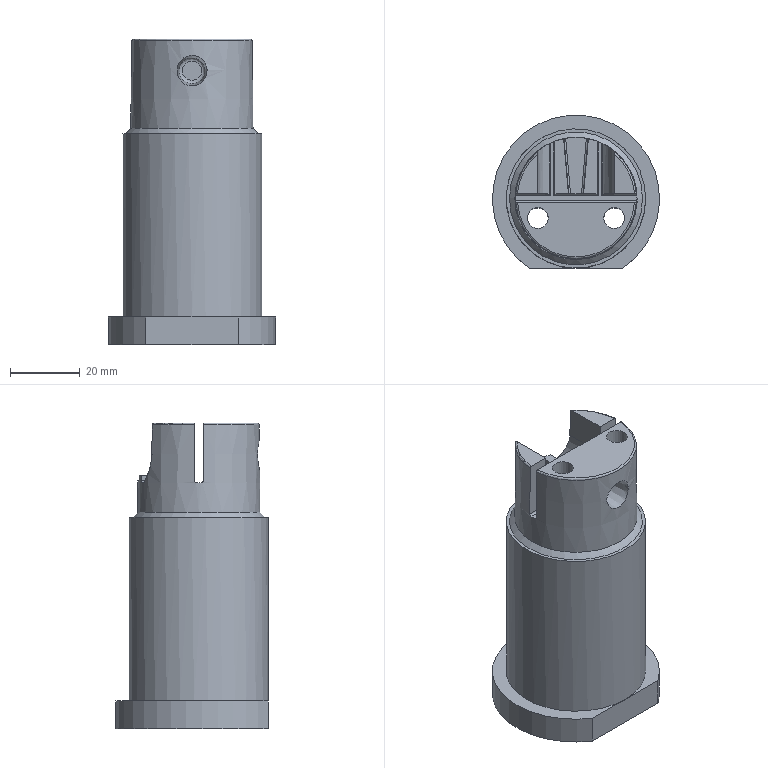Part | NX | features solid 2 | 1 solid | 47 faces | box 48 x 44 x 87.77 mm | volume 89878 mm3 | plane 21 | cylinder 17 | torus 4 | cone 3 | spline 2 | commonest cylinder face diameters 1.005 x8 1 x2 6 x2 22.11 x2 10 x1 40 x1
STEP:
#1=CARTESIAN_POINT('',(-13.266,-20.,-70.));
#2=VERTEX_POINT('',#1);
#3=CARTESIAN_POINT('',(13.266,-20.,-70.));
#4=VERTEX_POINT('',#3);
#5=CARTESIAN_POINT('',(0.,-20.,-70.));
#6=DIRECTION('',(1.,0.,0.));
#7=VECTOR('',#6,1000.);
#8=LINE('',#5,#7);
#9=EDGE_CURVE('',#2,#4,#8,.T.);
#10=ORIENTED_EDGE('',*,*,#9,.F.);
#11=CARTESIAN_POINT('',(0.,0.,-70.));
#12=DIRECTION('',(0.,0.,-1.));
#13=DIRECTION('',(-1.,0.,0.));
#14=AXIS2_PLACEMENT_3D('',#11,#12,#13);
#15=CIRCLE('',#14,24.);
#16=EDGE_CURVE('',#2,#4,#15,.T.);
#17=ORIENTED_EDGE('',*,*,#16,.T.);
#18=EDGE_LOOP('',(#10,#17));
#19=FACE_BOUND('',#18,.T.);
#20=CARTESIAN_POINT('',(7.98,-5.66,-70.));
#21=VERTEX_POINT('',#20);
#22=CARTESIAN_POINT('',(10.98,-5.66,-70.));
#23=DIRECTION('',(0.,0.,-1.));
#24=DIRECTION('',(-1.,0.,0.));
#25=AXIS2_PLACEMENT_3D('',#22,#23,#24);
#26=CIRCLE('',#25,3.);
#27=EDGE_CURVE('',#21,#21,#26,.T.);
#28=ORIENTED_EDGE('',*,*,#27,.F.);
#29=EDGE_LOOP('',(#28));
#30=FACE_BOUND('',#29,.T.);
#31=CARTESIAN_POINT('',(-13.98,-5.66,-70.));
#32=VERTEX_POINT('',#31);
#33=CARTESIAN_POINT('',(-10.98,-5.66,-70.));
#34=DIRECTION('',(0.,0.,-1.));
#35=DIRECTION('',(-1.,0.,0.));
#36=AXIS2_PLACEMENT_3D('',#33,#34,#35);
#37=CIRCLE('',#36,3.);
#38=EDGE_CURVE('',#32,#32,#37,.T.);
#39=ORIENTED_EDGE('',*,*,#38,.F.);
#40=EDGE_LOOP('',(#39));
#41=FACE_BOUND('',#40,.T.);
#42=CARTESIAN_POINT('',(-5.,7.,-70.));
#43=VERTEX_POINT('',#42);
#44=CARTESIAN_POINT('',(0.,7.,-70.));
#45=DIRECTION('',(0.,0.,-1.));
#46=DIRECTION('',(-1.,0.,0.));
#47=AXIS2_PLACEMENT_3D('',#44,#45,#46);
#48=CIRCLE('',#47,5.);
#49=EDGE_CURVE('',#43,#43,#48,.F.);
#50=ORIENTED_EDGE('',*,*,#49,.T.);
#51=EDGE_LOOP('',(#50));
#52=FACE_BOUND('',#51,.T.);
#53=CARTESIAN_POINT('',(0.,0.,-70.));
#54=DIRECTION('',(0.,0.,-1.));
#55=DIRECTION('',(-1.,0.,0.));
#56=AXIS2_PLACEMENT_3D('',#53,#54,#55);
#57=PLANE('',#56);
#58=ADVANCED_FACE('',(#19,#30,#41,#52),#57,.T.);
#59=CARTESIAN_POINT('',(0.,-20.,-62.));
#60=VERTEX_POINT('',#59);
#61=CARTESIAN_POINT('',(0.,0.,-62.));
#62=DIRECTION('',(0.,0.,-1.));
#63=DIRECTION('',(-1.,0.,0.));
#64=AXIS2_PLACEMENT_3D('',#61,#62,#63);
#65=CIRCLE('',#64,20.);
#66=EDGE_CURVE('',#60,#60,#65,.F.);
#67=ORIENTED_EDGE('',*,*,#66,.T.);
#68=EDGE_LOOP('',(#67));
#69=FACE_BOUND('',#68,.T.);
#70=CARTESIAN_POINT('',(20.,0.,-9.365));
#71=VERTEX_POINT('',#70);
#72=CARTESIAN_POINT('',(0.,0.,-9.365));
#73=DIRECTION('',(0.,0.,1.));
#74=DIRECTION('',(1.,0.,0.));
#75=AXIS2_PLACEMENT_3D('',#72,#73,#74);
#76=CIRCLE('',#75,20.);
#77=EDGE_CURVE('',#71,#71,#76,.F.);
#78=ORIENTED_EDGE('',*,*,#77,.T.);
#79=EDGE_LOOP('',(#78));
#80=FACE_BOUND('',#79,.T.);
#81=CARTESIAN_POINT('',(0.,0.,-104.365));
#82=DIRECTION('',(0.,0.,1.));
#83=DIRECTION('',(1.,0.,0.));
#84=AXIS2_PLACEMENT_3D('',#81,#82,#83);
#85=CYLINDRICAL_SURFACE('',#84,20.);
#86=ADVANCED_FACE('',(#69,#80),#85,.T.);
#87=CARTESIAN_POINT('',(0.,-9.452,11.49));
#88=VERTEX_POINT('',#87);
#89=CARTESIAN_POINT('',(0.,-9.452,8.725));
#90=DIRECTION('',(0.,1.,0.));
#91=DIRECTION('',(0.,0.,1.));
#92=AXIS2_PLACEMENT_3D('',#89,#90,#91);
#93=CIRCLE('',#92,2.764);
#94=EDGE_CURVE('',#88,#88,#93,.F.);
#95=ORIENTED_EDGE('',*,*,#94,.T.);
#96=EDGE_LOOP('',(#95));
#97=FACE_BOUND('',#96,.T.);
#98=CARTESIAN_POINT('',(0.,-9.452,8.725));
#99=DIRECTION('',(0.,1.,0.));
#100=DIRECTION('',(0.,0.,1.));
#101=AXIS2_PLACEMENT_3D('',#98,#99,#100);
#102=PLANE('',#101);
#103=ADVANCED_FACE('',(#97),#102,.F.);
#104=CARTESIAN_POINT('',(0.,-10.364,12.486));
#105=VERTEX_POINT('',#104);
#106=CARTESIAN_POINT('',(0.,-10.364,8.725));
#107=DIRECTION('',(0.,1.,0.));
#108=DIRECTION('',(0.,0.,1.));
#109=AXIS2_PLACEMENT_3D('',#106,#107,#108);
#110=CIRCLE('',#109,3.761);
#111=EDGE_CURVE('',#105,#105,#110,.T.);
#112=ORIENTED_EDGE('',*,*,#111,.F.);
#113=EDGE_LOOP('',(#112));
#114=FACE_BOUND('',#113,.T.);
#115=ORIENTED_EDGE('',*,*,#94,.F.);
#116=EDGE_LOOP('',(#115));
#117=FACE_BOUND('',#116,.T.);
#118=CARTESIAN_POINT('',(0.,-10.452,8.725));
#119=DIRECTION('',(0.,1.,0.));
#120=DIRECTION('',(0.,0.,1.));
#121=AXIS2_PLACEMENT_3D('',#118,#119,#120);
#122=TOROIDAL_SURFACE('',#121,2.764,1.);
#123=ADVANCED_FACE('',(#114,#117),#122,.F.);
#124=CARTESIAN_POINT('',(-11.055,12.72,17.77));
#125=VERTEX_POINT('',#124);
#126=CARTESIAN_POINT('',(-11.055,1.256,17.77));
#127=VERTEX_POINT('',#126);
#128=CARTESIAN_POINT('',(-11.055,1.256,17.77));
#129=DIRECTION('',(0.,1.,0.));
#130=VECTOR('',#129,1000.);
#131=LINE('',#128,#130);
#132=EDGE_CURVE('',#125,#127,#131,.F.);
#133=ORIENTED_EDGE('',*,*,#132,.F.);
#134=CARTESIAN_POINT('',(-16.806,1.256,17.77));
#135=VERTEX_POINT('',#134);
#136=CARTESIAN_POINT('',(0.,0.,17.77));
#137=DIRECTION('',(0.,0.,1.));
#138=DIRECTION('',(-0.656,0.7548,0.));
#139=AXIS2_PLACEMENT_3D('',#136,#137,#138);
#140=CIRCLE('',#139,16.853);
#141=EDGE_CURVE('',#135,#125,#140,.F.);
#142=ORIENTED_EDGE('',*,*,#141,.F.);
#143=CARTESIAN_POINT('',(-11.055,1.256,17.77));
#144=DIRECTION('',(-1.,0.,0.));
#145=VECTOR('',#144,1000.);
#146=LINE('',#143,#145);
#147=EDGE_CURVE('',#135,#127,#146,.F.);
#148=ORIENTED_EDGE('',*,*,#147,.T.);
#149=EDGE_LOOP('',(#133,#142,#148));
#150=FACE_BOUND('',#149,.T.);
#151=CARTESIAN_POINT('',(0.,0.,17.77));
#152=DIRECTION('',(0.,0.,-1.));
#153=DIRECTION('',(1.,0.,0.));
#154=AXIS2_PLACEMENT_3D('',#151,#152,#153);
#155=PLANE('',#154);
#156=ADVANCED_FACE('',(#150),#155,.F.);
#157=CARTESIAN_POINT('',(-13.98,-5.66,17.77));
#158=VERTEX_POINT('',#157);
#159=CARTESIAN_POINT('',(-10.98,-5.66,17.77));
#160=DIRECTION('',(0.,0.,-1.));
#161=DIRECTION('',(-1.,0.,0.));
#162=AXIS2_PLACEMENT_3D('',#159,#160,#161);
#163=CIRCLE('',#162,3.);
#164=EDGE_CURVE('',#158,#158,#163,.T.);
#165=ORIENTED_EDGE('',*,*,#164,.T.);
#166=EDGE_LOOP('',(#165));
#167=FACE_BOUND('',#166,.T.);
#168=CARTESIAN_POINT('',(7.98,-5.66,17.77));
#169=VERTEX_POINT('',#168);
#170=CARTESIAN_POINT('',(10.98,-5.66,17.77));
#171=DIRECTION('',(0.,0.,-1.));
#172=DIRECTION('',(-1.,0.,0.));
#173=AXIS2_PLACEMENT_3D('',#170,#171,#172);
#174=CIRCLE('',#173,3.);
#175=EDGE_CURVE('',#169,#169,#174,.T.);
#176=ORIENTED_EDGE('',*,*,#175,.T.);
#177=EDGE_LOOP('',(#176));
#178=FACE_BOUND('',#177,.T.);
#179=CARTESIAN_POINT('',(-16.806,-1.256,17.77));
#180=VERTEX_POINT('',#179);
#181=CARTESIAN_POINT('',(16.806,-1.256,17.77));
#182=VERTEX_POINT('',#181);
#183=CARTESIAN_POINT('',(16.806,-1.256,17.77));
#184=DIRECTION('',(-1.,0.,0.));
#185=VECTOR('',#184,1000.);
#186=LINE('',#183,#185);
#187=EDGE_CURVE('',#180,#182,#186,.F.);
#188=ORIENTED_EDGE('',*,*,#187,.F.);
#189=CARTESIAN_POINT('',(0.,0.,17.77));
#190=DIRECTION('',(0.,0.,1.));
#191=DIRECTION('',(-0.9972,-0.07454,0.));
#192=AXIS2_PLACEMENT_3D('',#189,#190,#191);
#193=CIRCLE('',#192,16.853);
#194=EDGE_CURVE('',#182,#180,#193,.F.);
#195=ORIENTED_EDGE('',*,*,#194,.F.);
#196=EDGE_LOOP('',(#188,#195));
#197=FACE_BOUND('',#196,.T.);
#198=CARTESIAN_POINT('',(0.,0.,17.77));
#199=DIRECTION('',(0.,0.,-1.));
#200=DIRECTION('',(1.,0.,0.));
#201=AXIS2_PLACEMENT_3D('',#198,#199,#200);
#202=PLANE('',#201);
#203=ADVANCED_FACE('',(#167,#178,#197),#202,.F.);
#204=CARTESIAN_POINT('',(11.055,1.256,17.77));
#205=VERTEX_POINT('',#204);
#206=CARTESIAN_POINT('',(16.806,1.256,17.77));
#207=VERTEX_POINT('',#206);
#208=CARTESIAN_POINT('',(16.806,1.256,17.77));
#209=DIRECTION('',(-1.,0.,0.));
#210=VECTOR('',#209,1000.);
#211=LINE('',#208,#210);
#212=EDGE_CURVE('',#205,#207,#211,.F.);
#213=ORIENTED_EDGE('',*,*,#212,.T.);
#214=CARTESIAN_POINT('',(11.055,12.72,17.77));
#215=VERTEX_POINT('',#214);
#216=CARTESIAN_POINT('',(0.,0.,17.77));
#217=DIRECTION('',(0.,0.,1.));
#218=DIRECTION('',(0.9972,0.07454,0.));
#219=AXIS2_PLACEMENT_3D('',#216,#217,#218);
#220=CIRCLE('',#219,16.853);
#221=EDGE_CURVE('',#215,#207,#220,.F.);
#222=ORIENTED_EDGE('',*,*,#221,.F.);
#223=CARTESIAN_POINT('',(11.055,12.72,17.77));
#224=DIRECTION('',(0.,-1.,0.));
#225=VECTOR('',#224,1000.);
#226=LINE('',#223,#225);
#227=EDGE_CURVE('',#205,#215,#226,.F.);
#228=ORIENTED_EDGE('',*,*,#227,.F.);
#229=EDGE_LOOP('',(#213,#222,#228));
#230=FACE_BOUND('',#229,.T.);
#231=CARTESIAN_POINT('',(0.,0.,17.77));
#232=DIRECTION('',(0.,0.,-1.));
#233=DIRECTION('',(1.,0.,0.));
#234=AXIS2_PLACEMENT_3D('',#231,#232,#233);
#235=PLANE('',#234);
#236=ADVANCED_FACE('',(#230),#235,.F.);
#237=CARTESIAN_POINT('',(-6.03,1.256,1.188));
#238=VERTEX_POINT('',#237);
#239=CARTESIAN_POINT('',(6.03,1.256,1.188));
#240=VERTEX_POINT('',#239);
#241=CARTESIAN_POINT('',(6.03,1.256,1.188));
#242=DIRECTION('',(-1.,0.,0.));
#243=VECTOR('',#242,1000.);
#244=LINE('',#241,#243);
#245=EDGE_CURVE('',#238,#240,#244,.F.);
#246=ORIENTED_EDGE('',*,*,#245,.F.);
#247=CARTESIAN_POINT('',(-6.532,0.7538,0.6852));
#248=VERTEX_POINT('',#247);
#249=CARTESIAN_POINT('',(-6.532,0.7538,1.188));
#250=DIRECTION('',(-0.7071,0.7071,0.));
#251=DIRECTION('',(-0.7071,-0.7071,0.));
#252=AXIS2_PLACEMENT_3D('',#249,#250,#251);
#253=ELLIPSE('',#252,0.7106,0.5025);
#254=EDGE_CURVE('',#248,#238,#253,.F.);
#255=ORIENTED_EDGE('',*,*,#254,.F.);
#256=CARTESIAN_POINT('',(6.532,0.7538,0.6852));
#257=VERTEX_POINT('',#256);
#258=CARTESIAN_POINT('',(6.532,0.7538,0.6852));
#259=DIRECTION('',(-1.,0.,0.));
#260=VECTOR('',#259,1000.);
#261=LINE('',#258,#260);
#262=EDGE_CURVE('',#248,#257,#261,.F.);
#263=ORIENTED_EDGE('',*,*,#262,.T.);
#264=CARTESIAN_POINT('',(6.532,0.7538,1.188));
#265=DIRECTION('',(-0.7071,-0.7071,0.));
#266=DIRECTION('',(-0.7071,0.7071,0.));
#267=AXIS2_PLACEMENT_3D('',#264,#265,#266);
#268=ELLIPSE('',#267,0.7106,0.5025);
#269=EDGE_CURVE('',#240,#257,#268,.T.);
#270=ORIENTED_EDGE('',*,*,#269,.F.);
#271=EDGE_LOOP('',(#246,#255,#263,#270));
#272=FACE_BOUND('',#271,.T.);
#273=CARTESIAN_POINT('',(196.261,0.7538,1.188));
#274=DIRECTION('',(-1.,0.,0.));
#275=DIRECTION('',(0.,-1.,0.));
#276=AXIS2_PLACEMENT_3D('',#273,#274,#275);
#277=CYLINDRICAL_SURFACE('',#276,0.5025);
#278=ADVANCED_FACE('',(#272),#277,.F.);
#279=CARTESIAN_POINT('',(-2.07,1.256,1.656));
#280=VERTEX_POINT('',#279);
#281=CARTESIAN_POINT('',(-1.57,1.256,1.2));
#282=VERTEX_POINT('',#281);
#283=CARTESIAN_POINT('',(-1.57,1.256,1.7));
#284=DIRECTION('',(0.,1.,0.));
#285=DIRECTION('',(1.,0.,0.));
#286=AXIS2_PLACEMENT_3D('',#283,#284,#285);
#287=ELLIPSE('',#286,0.5019,0.5);
#288=EDGE_CURVE('',#280,#282,#287,.F.);
#289=ORIENTED_EDGE('',*,*,#288,.F.);
#290=CARTESIAN_POINT('',(-2.188,1.256,3.004));
#291=VERTEX_POINT('',#290);
#292=CARTESIAN_POINT('',(-2.03,1.256,1.2));
#293=DIRECTION('',(-0.08749,0.,0.9962));
#294=VECTOR('',#293,1000.);
#295=LINE('',#292,#294);
#296=EDGE_CURVE('',#280,#291,#295,.T.);
#297=ORIENTED_EDGE('',*,*,#296,.T.);
#298=CARTESIAN_POINT('',(-6.03,1.256,3.004));
#299=VERTEX_POINT('',#298);
#300=CARTESIAN_POINT('',(0.,1.256,3.004));
#301=DIRECTION('',(-1.,0.,0.));
#302=VECTOR('',#301,1000.);
#303=LINE('',#300,#302);
#304=EDGE_CURVE('',#291,#299,#303,.T.);
#305=ORIENTED_EDGE('',*,*,#304,.T.);
#306=CARTESIAN_POINT('',(-6.03,1.256,1.188));
#307=DIRECTION('',(0.,0.,1.));
#308=VECTOR('',#307,1000.);
#309=LINE('',#306,#308);
#310=EDGE_CURVE('',#299,#238,#309,.F.);
#311=ORIENTED_EDGE('',*,*,#310,.T.);
#312=ORIENTED_EDGE('',*,*,#245,.T.);
#313=CARTESIAN_POINT('',(6.03,1.256,3.004));
#314=VERTEX_POINT('',#313);
#315=CARTESIAN_POINT('',(6.03,1.256,1.188));
#316=DIRECTION('',(0.,0.,1.));
#317=VECTOR('',#316,1000.);
#318=LINE('',#315,#317);
#319=EDGE_CURVE('',#314,#240,#318,.F.);
#320=ORIENTED_EDGE('',*,*,#319,.F.);
#321=CARTESIAN_POINT('',(2.188,1.256,3.004));
#322=VERTEX_POINT('',#321);
#323=CARTESIAN_POINT('',(0.,1.256,3.004));
#324=DIRECTION('',(-1.,0.,0.));
#325=VECTOR('',#324,1000.);
#326=LINE('',#323,#325);
#327=EDGE_CURVE('',#314,#322,#326,.T.);
#328=ORIENTED_EDGE('',*,*,#327,.T.);
#329=CARTESIAN_POINT('',(2.07,1.256,1.656));
#330=VERTEX_POINT('',#329);
#331=CARTESIAN_POINT('',(1.997,1.256,0.8247));
#332=DIRECTION('',(0.08749,0.,0.9962));
#333=VECTOR('',#332,1000.);
#334=LINE('',#331,#333);
#335=EDGE_CURVE('',#330,#322,#334,.T.);
#336=ORIENTED_EDGE('',*,*,#335,.F.);
#337=CARTESIAN_POINT('',(1.57,1.256,1.2));
#338=VERTEX_POINT('',#337);
#339=CARTESIAN_POINT('',(1.57,1.256,1.7));
#340=DIRECTION('',(0.,1.,0.));
#341=DIRECTION('',(1.,0.,0.));
#342=AXIS2_PLACEMENT_3D('',#339,#340,#341);
#343=ELLIPSE('',#342,0.5019,0.5);
#344=EDGE_CURVE('',#338,#330,#343,.F.);
#345=ORIENTED_EDGE('',*,*,#344,.F.);
#346=CARTESIAN_POINT('',(0.,1.256,1.2));
#347=DIRECTION('',(1.,0.,0.));
#348=VECTOR('',#347,1000.);
#349=LINE('',#346,#348);
#350=EDGE_CURVE('',#282,#338,#349,.T.);
#351=ORIENTED_EDGE('',*,*,#350,.F.);
#352=EDGE_LOOP('',(#289,#297,#305,#311,#312,#320,#328,#336,#345,#351));
#353=FACE_BOUND('',#352,.T.);
#354=CARTESIAN_POINT('',(-18.15,1.256,17.77));
#355=DIRECTION('',(0.,1.,0.));
#356=DIRECTION('',(-1.,0.,0.));
#357=AXIS2_PLACEMENT_3D('',#354,#355,#356);
#358=PLANE('',#357);
#359=ADVANCED_FACE('',(#353),#358,.F.);
#360=ORIENTED_EDGE('',*,*,#111,.T.);
#361=EDGE_LOOP('',(#360));
#362=FACE_BOUND('',#361,.T.);
#363=CARTESIAN_POINT('',(-3.148,-17.17,5.715));
#364=VERTEX_POINT('',#363);
#365=CARTESIAN_POINT('',(-0.1207,-17.607,3.863));
#366=CARTESIAN_POINT('',(-3.495,-17.166,5.395));
#367=CARTESIAN_POINT('',(-4.79,-16.745,8.843));
#368=CARTESIAN_POINT('',(-3.323,-17.147,12.223));
#369=CARTESIAN_POINT('',(0.1224,-17.523,13.581));
#370=CARTESIAN_POINT('',(3.495,-17.107,12.048));
#371=CARTESIAN_POINT('',(4.79,-16.747,8.598));
#372=CARTESIAN_POINT('',(3.32,-17.21,5.218));
#373=CARTESIAN_POINT('',(-0.1207,-17.607,3.863));
#374=CARTESIAN_POINT('',(-3.495,-17.166,5.395));
#375=CARTESIAN_POINT('',(-4.79,-16.745,8.843));
#376=B_SPLINE_CURVE_WITH_KNOTS('',3,(#365,#366,#367,#368,#369,#370,#371,#372,#373,#374,#375),.UNSPECIFIED.,.T.,.F.,(1,1,1,1,1,1,1,1,1,1,1,1,1,1,1),(-0.01025,-0.006833,-0.003417,0.,0.003417,0.006833,0.01025,0.01367,0.01708,0.0205,0.02392,0.02733,0.03075,0.03417,0.03758),.UNSPECIFIED.);
#377=EDGE_CURVE('',#364,#364,#376,.T.);
#378=ORIENTED_EDGE('',*,*,#377,.F.);
#379=EDGE_LOOP('',(#378));
#380=FACE_BOUND('',#379,.T.);
#381=CARTESIAN_POINT('',(0.,-13.8,8.725));
#382=DIRECTION('',(0.,-1.,0.));
#383=DIRECTION('',(0.,0.,1.));
#384=AXIS2_PLACEMENT_3D('',#381,#382,#383);
#385=CONICAL_SURFACE('',#384,4.061,0.08727);
#386=ADVANCED_FACE('',(#362,#380),#385,.F.);
#387=ORIENTED_EDGE('',*,*,#335,.T.);
#388=CARTESIAN_POINT('',(3.558,17.115,2.805));
#389=VERTEX_POINT('',#388);
#390=CARTESIAN_POINT('',(2.188,1.256,3.004));
#391=CARTESIAN_POINT('',(2.645,6.543,2.937));
#392=CARTESIAN_POINT('',(3.102,11.829,2.87));
#393=CARTESIAN_POINT('',(3.558,17.115,2.805));
#394=B_SPLINE_CURVE_WITH_KNOTS('',3,(#390,#391,#392,#393),.UNSPECIFIED.,.F.,.F.,(4,4),(0.,0.01592),.UNSPECIFIED.);
#395=EDGE_CURVE('',#322,#389,#394,.T.);
#396=ORIENTED_EDGE('',*,*,#395,.T.);
#397=CARTESIAN_POINT('',(3.46,17.146,1.656));
#398=VERTEX_POINT('',#397);
#399=CARTESIAN_POINT('',(-1.775,0.1553,-41.03));
#400=DIRECTION('',(0.9924,-0.08682,-0.08716));
#401=DIRECTION('',(-0.08682,0.007596,-0.9962));
#402=AXIS2_PLACEMENT_3D('',#399,#400,#401);
#403=ELLIPSE('',#402,204.965,17.775);
#404=EDGE_CURVE('',#398,#389,#403,.T.);
#405=ORIENTED_EDGE('',*,*,#404,.F.);
#406=CARTESIAN_POINT('',(2.07,1.253,1.656));
#407=DIRECTION('',(0.08716,0.9962,0.));
#408=VECTOR('',#407,1000.);
#409=LINE('',#406,#408);
#410=EDGE_CURVE('',#398,#330,#409,.F.);
#411=ORIENTED_EDGE('',*,*,#410,.T.);
#412=EDGE_LOOP('',(#387,#396,#405,#411));
#413=FACE_BOUND('',#412,.T.);
#414=CARTESIAN_POINT('',(2.03,1.256,1.2));
#415=DIRECTION('',(0.9924,-0.08682,-0.08716));
#416=DIRECTION('',(-0.08749,0.,-0.9962));
#417=AXIS2_PLACEMENT_3D('',#414,#415,#416);
#418=PLANE('',#417);
#419=ADVANCED_FACE('',(#413),#418,.F.);
#420=ORIENTED_EDGE('',*,*,#344,.T.);
#421=ORIENTED_EDGE('',*,*,#410,.F.);
#422=CARTESIAN_POINT('',(2.969,17.242,1.2));
#423=VERTEX_POINT('',#422);
#424=CARTESIAN_POINT('',(3.46,17.146,1.656));
#425=CARTESIAN_POINT('',(3.439,17.152,1.407));
#426=CARTESIAN_POINT('',(3.215,17.199,1.2));
#427=CARTESIAN_POINT('',(2.969,17.242,1.2));
#428=B_SPLINE_CURVE_WITH_KNOTS('',3,(#424,#425,#426,#427),.UNSPECIFIED.,.F.,.F.,(4,4),(0.,0.0007397),.UNSPECIFIED.);
#429=EDGE_CURVE('',#398,#423,#428,.T.);
#430=ORIENTED_EDGE('',*,*,#429,.T.);
#431=CARTESIAN_POINT('',(2.263,9.171,1.2));
#432=DIRECTION('',(0.08716,0.9962,0.));
#433=VECTOR('',#432,1000.);
#434=LINE('',#431,#433);
#435=EDGE_CURVE('',#338,#423,#434,.T.);
#436=ORIENTED_EDGE('',*,*,#435,.F.);
#437=EDGE_LOOP('',(#420,#421,#430,#436));
#438=FACE_BOUND('',#437,.T.);
#439=CARTESIAN_POINT('',(1.574,1.296,1.7));
#440=DIRECTION('',(0.08716,0.9962,0.));
#441=DIRECTION('',(-0.9962,0.08716,0.));
#442=AXIS2_PLACEMENT_3D('',#439,#440,#441);
#443=CYLINDRICAL_SURFACE('',#442,0.5);
#444=ADVANCED_FACE('',(#438),#443,.F.);
#445=ORIENTED_EDGE('',*,*,#350,.T.);
#446=ORIENTED_EDGE('',*,*,#435,.T.);
#447=CARTESIAN_POINT('',(-2.969,17.242,1.2));
#448=VERTEX_POINT('',#447);
#449=CARTESIAN_POINT('',(0.,0.,1.2));
#450=DIRECTION('',(0.,0.,-1.));
#451=DIRECTION('',(-1.,0.,0.));
#452=AXIS2_PLACEMENT_3D('',#449,#450,#451);
#453=CIRCLE('',#452,17.495);
#454=EDGE_CURVE('',#448,#423,#453,.T.);
#455=ORIENTED_EDGE('',*,*,#454,.F.);
#456=CARTESIAN_POINT('',(-2.263,9.171,1.2));
#457=DIRECTION('',(0.08716,-0.9962,0.));
#458=VECTOR('',#457,1000.);
#459=LINE('',#456,#458);
#460=EDGE_CURVE('',#448,#282,#459,.T.);
#461=ORIENTED_EDGE('',*,*,#460,.T.);
#462=EDGE_LOOP('',(#445,#446,#455,#461));
#463=FACE_BOUND('',#462,.T.);
#464=CARTESIAN_POINT('',(0.,9.369,1.2));
#465=DIRECTION('',(0.,0.,-1.));
#466=DIRECTION('',(-1.,0.,0.));
#467=AXIS2_PLACEMENT_3D('',#464,#465,#466);
#468=PLANE('',#467);
#469=ADVANCED_FACE('',(#463),#468,.F.);
#470=CARTESIAN_POINT('',(-3.46,17.146,1.656));
#471=VERTEX_POINT('',#470);
#472=CARTESIAN_POINT('',(-2.969,17.242,1.2));
#473=CARTESIAN_POINT('',(-3.215,17.199,1.2));
#474=CARTESIAN_POINT('',(-3.439,17.152,1.407));
#475=CARTESIAN_POINT('',(-3.46,17.146,1.656));
#476=B_SPLINE_CURVE_WITH_KNOTS('',3,(#472,#473,#474,#475),.UNSPECIFIED.,.F.,.F.,(4,4),(0.,0.0007398),.UNSPECIFIED.);
#477=EDGE_CURVE('',#448,#471,#476,.T.);
#478=ORIENTED_EDGE('',*,*,#477,.T.);
#479=CARTESIAN_POINT('',(-2.07,1.253,1.656));
#480=DIRECTION('',(0.08716,-0.9962,0.));
#481=VECTOR('',#480,1000.);
#482=LINE('',#479,#481);
#483=EDGE_CURVE('',#280,#471,#482,.F.);
#484=ORIENTED_EDGE('',*,*,#483,.F.);
#485=ORIENTED_EDGE('',*,*,#288,.T.);
#486=ORIENTED_EDGE('',*,*,#460,.F.);
#487=EDGE_LOOP('',(#478,#484,#485,#486));
#488=FACE_BOUND('',#487,.T.);
#489=CARTESIAN_POINT('',(-1.574,1.296,1.7));
#490=DIRECTION('',(0.08716,-0.9962,0.));
#491=DIRECTION('',(0.9962,0.08716,0.));
#492=AXIS2_PLACEMENT_3D('',#489,#490,#491);
#493=CYLINDRICAL_SURFACE('',#492,0.5);
#494=ADVANCED_FACE('',(#488),#493,.F.);
#495=CARTESIAN_POINT('',(-3.558,17.115,2.805));
#496=VERTEX_POINT('',#495);
#497=CARTESIAN_POINT('',(1.775,0.1553,-41.03));
#498=DIRECTION('',(-0.9924,-0.08682,-0.08716));
#499=DIRECTION('',(0.08682,0.007596,-0.9962));
#500=AXIS2_PLACEMENT_3D('',#497,#498,#499);
#501=ELLIPSE('',#500,204.965,17.775);
#502=EDGE_CURVE('',#496,#471,#501,.T.);
#503=ORIENTED_EDGE('',*,*,#502,.F.);
#504=CARTESIAN_POINT('',(-3.558,17.115,2.805));
#505=CARTESIAN_POINT('',(-3.102,11.829,2.87));
#506=CARTESIAN_POINT('',(-2.645,6.543,2.937));
#507=CARTESIAN_POINT('',(-2.188,1.256,3.004));
#508=B_SPLINE_CURVE_WITH_KNOTS('',3,(#504,#505,#506,#507),.UNSPECIFIED.,.F.,.F.,(4,4),(0.0003674,0.01629),.UNSPECIFIED.);
#509=EDGE_CURVE('',#496,#291,#508,.T.);
#510=ORIENTED_EDGE('',*,*,#509,.T.);
#511=ORIENTED_EDGE('',*,*,#296,.F.);
#512=ORIENTED_EDGE('',*,*,#483,.T.);
#513=EDGE_LOOP('',(#503,#510,#511,#512));
#514=FACE_BOUND('',#513,.T.);
#515=CARTESIAN_POINT('',(-2.03,1.256,1.2));
#516=DIRECTION('',(-0.9924,-0.08682,-0.08716));
#517=DIRECTION('',(-0.08749,0.,0.9962));
#518=AXIS2_PLACEMENT_3D('',#515,#516,#517);
#519=PLANE('',#518);
#520=ADVANCED_FACE('',(#514),#519,.F.);
#521=ORIENTED_EDGE('',*,*,#509,.F.);
#522=CARTESIAN_POINT('',(-6.03,16.408,2.813));
#523=VERTEX_POINT('',#522);
#524=CARTESIAN_POINT('',(-6.03,16.408,2.813));
#525=CARTESIAN_POINT('',(-5.217,16.707,2.81));
#526=CARTESIAN_POINT('',(-4.393,16.942,2.807));
#527=CARTESIAN_POINT('',(-3.558,17.115,2.805));
#528=B_SPLINE_CURVE_WITH_KNOTS('',3,(#524,#525,#526,#527),.UNSPECIFIED.,.F.,.F.,(4,4),(0.,0.002557),.UNSPECIFIED.);
#529=EDGE_CURVE('',#523,#496,#528,.T.);
#530=ORIENTED_EDGE('',*,*,#529,.F.);
#531=CARTESIAN_POINT('',(-6.03,1.256,3.004));
#532=CARTESIAN_POINT('',(-6.03,6.307,2.94));
#533=CARTESIAN_POINT('',(-6.03,11.358,2.876));
#534=CARTESIAN_POINT('',(-6.03,16.408,2.813));
#535=B_SPLINE_CURVE_WITH_KNOTS('',3,(#531,#532,#533,#534),.UNSPECIFIED.,.F.,.F.,(4,4),(0.,1.),.PIECEWISE_BEZIER_KNOTS.);
#536=EDGE_CURVE('',#523,#299,#535,.F.);
#537=ORIENTED_EDGE('',*,*,#536,.T.);
#538=ORIENTED_EDGE('',*,*,#304,.F.);
#539=EDGE_LOOP('',(#521,#530,#537,#538));
#540=FACE_BOUND('',#539,.T.);
#541=CARTESIAN_POINT('',(-2.165,17.21,2.803));
#542=CARTESIAN_POINT('',(-6.03,17.21,2.803));
#543=CARTESIAN_POINT('',(-2.165,16.943,2.807));
#544=CARTESIAN_POINT('',(-6.03,16.943,2.807));
#545=CARTESIAN_POINT('',(-2.165,11.625,2.873));
#546=CARTESIAN_POINT('',(-6.03,11.625,2.873));
#547=CARTESIAN_POINT('',(-2.165,6.307,2.94));
#548=CARTESIAN_POINT('',(-6.03,6.307,2.94));
#549=CARTESIAN_POINT('',(-2.165,1.256,3.004));
#550=CARTESIAN_POINT('',(-6.03,1.256,3.004));
#551=B_SPLINE_SURFACE_WITH_KNOTS('',3,1,((#541,#542),(#543,#544),(#545,#546),(#547,#548),(#549,#550)),.SURF_OF_LINEAR_EXTRUSION.,.F.,.F.,.F.,(4,1,4),(2,2),(-0.05294,0.,1.),(0.6795,1.),.UNSPECIFIED.);
#552=ADVANCED_FACE('',(#540),#551,.F.);
#553=CARTESIAN_POINT('',(-6.03,16.423,1.188));
#554=VERTEX_POINT('',#553);
#555=CARTESIAN_POINT('',(-6.03,16.408,2.813));
#556=CARTESIAN_POINT('',(-6.03,16.413,2.272));
#557=CARTESIAN_POINT('',(-6.03,16.418,1.73));
#558=CARTESIAN_POINT('',(-6.03,16.423,1.188));
#559=B_SPLINE_CURVE_WITH_KNOTS('',3,(#555,#556,#557,#558),.UNSPECIFIED.,.F.,.F.,(4,4),(0.,1.),.PIECEWISE_BEZIER_KNOTS.);
#560=EDGE_CURVE('',#554,#523,#559,.F.);
#561=ORIENTED_EDGE('',*,*,#560,.F.);
#562=CARTESIAN_POINT('',(-6.03,1.256,1.188));
#563=DIRECTION('',(0.,1.,0.));
#564=VECTOR('',#563,1000.);
#565=LINE('',#562,#564);
#566=EDGE_CURVE('',#554,#238,#565,.F.);
#567=ORIENTED_EDGE('',*,*,#566,.T.);
#568=ORIENTED_EDGE('',*,*,#310,.F.);
#569=ORIENTED_EDGE('',*,*,#536,.F.);
#570=EDGE_LOOP('',(#561,#567,#568,#569));
#571=FACE_BOUND('',#570,.T.);
#572=CARTESIAN_POINT('',(-6.03,0.,-0.5405));
#573=DIRECTION('',(1.,0.,0.));
#574=DIRECTION('',(0.,0.,-1.));
#575=AXIS2_PLACEMENT_3D('',#572,#573,#574);
#576=PLANE('',#575);
#577=ADVANCED_FACE('',(#571),#576,.F.);
#578=CARTESIAN_POINT('',(-6.532,16.235,0.6852));
#579=VERTEX_POINT('',#578);
#580=CARTESIAN_POINT('',(-6.03,16.423,1.188));
#581=CARTESIAN_POINT('',(-6.03,16.426,0.9127));
#582=CARTESIAN_POINT('',(-6.278,16.337,0.6852));
#583=CARTESIAN_POINT('',(-6.532,16.235,0.6852));
#584=B_SPLINE_CURVE_WITH_KNOTS('',3,(#580,#581,#582,#583),.UNSPECIFIED.,.F.,.F.,(4,4),(0.,0.0008129),.UNSPECIFIED.);
#585=EDGE_CURVE('',#579,#554,#584,.F.);
#586=ORIENTED_EDGE('',*,*,#585,.F.);
#587=CARTESIAN_POINT('',(-6.532,16.235,0.6852));
#588=DIRECTION('',(0.,-1.,0.));
#589=VECTOR('',#588,1000.);
#590=LINE('',#587,#589);
#591=EDGE_CURVE('',#248,#579,#590,.F.);
#592=ORIENTED_EDGE('',*,*,#591,.F.);
#593=ORIENTED_EDGE('',*,*,#254,.T.);
#594=ORIENTED_EDGE('',*,*,#566,.F.);
#595=EDGE_LOOP('',(#586,#592,#593,#594));
#596=FACE_BOUND('',#595,.T.);
#597=CARTESIAN_POINT('',(-6.532,-212.801,1.188));
#598=DIRECTION('',(0.,1.,0.));
#599=DIRECTION('',(-1.,0.,0.));
#600=AXIS2_PLACEMENT_3D('',#597,#598,#599);
#601=CYLINDRICAL_SURFACE('',#600,0.5025);
#602=ADVANCED_FACE('',(#596),#601,.F.);
#603=CARTESIAN_POINT('',(-7.737,15.695,0.8288));
#604=VERTEX_POINT('',#603);
#605=CARTESIAN_POINT('',(-7.385,15.865,0.6852));
#606=VERTEX_POINT('',#605);
#607=CARTESIAN_POINT('',(-7.385,15.865,0.6852));
#608=CARTESIAN_POINT('',(-7.515,15.805,0.6852));
#609=CARTESIAN_POINT('',(-7.64,15.744,0.7343));
#610=CARTESIAN_POINT('',(-7.737,15.695,0.8288));
#611=B_SPLINE_CURVE_WITH_KNOTS('',3,(#607,#608,#609,#610),.UNSPECIFIED.,.F.,.F.,(4,4),(0.,0.0004236),.UNSPECIFIED.);
#612=EDGE_CURVE('',#604,#606,#611,.F.);
#613=ORIENTED_EDGE('',*,*,#612,.F.);
#614=CARTESIAN_POINT('',(-7.737,1.105,0.8288));
#615=VERTEX_POINT('',#614);
#616=CARTESIAN_POINT('',(-7.737,1.105,0.8288));
#617=DIRECTION('',(0.,1.,0.));
#618=VECTOR('',#617,1000.);
#619=LINE('',#616,#618);
#620=EDGE_CURVE('',#604,#615,#619,.F.);
#621=ORIENTED_EDGE('',*,*,#620,.T.);
#622=CARTESIAN_POINT('',(-7.385,0.7538,0.6852));
#623=VERTEX_POINT('',#622);
#624=CARTESIAN_POINT('',(-7.385,0.7538,1.188));
#625=DIRECTION('',(-0.7071,-0.7071,0.));
#626=DIRECTION('',(0.7071,-0.7071,0.));
#627=AXIS2_PLACEMENT_3D('',#624,#625,#626);
#628=ELLIPSE('',#627,0.7106,0.5025);
#629=EDGE_CURVE('',#623,#615,#628,.F.);
#630=ORIENTED_EDGE('',*,*,#629,.F.);
#631=CARTESIAN_POINT('',(-7.385,15.865,0.6852));
#632=DIRECTION('',(0.,-1.,0.));
#633=VECTOR('',#632,1000.);
#634=LINE('',#631,#633);
#635=EDGE_CURVE('',#623,#606,#634,.F.);
#636=ORIENTED_EDGE('',*,*,#635,.T.);
#637=EDGE_LOOP('',(#613,#621,#630,#636));
#638=FACE_BOUND('',#637,.T.);
#639=CARTESIAN_POINT('',(-7.385,227.196,1.188));
#640=DIRECTION('',(0.,-1.,0.));
#641=DIRECTION('',(0.6999,0.,0.7143));
#642=AXIS2_PLACEMENT_3D('',#639,#640,#641);
#643=CYLINDRICAL_SURFACE('',#642,0.5025);
#644=ADVANCED_FACE('',(#638),#643,.F.);
#645=CARTESIAN_POINT('',(-11.055,1.256,8.725));
#646=VERTEX_POINT('',#645);
#647=CARTESIAN_POINT('',(-11.055,13.475,8.725));
#648=VERTEX_POINT('',#647);
#649=CARTESIAN_POINT('',(-11.055,13.475,8.725));
#650=DIRECTION('',(0.,-1.,0.));
#651=VECTOR('',#650,1000.);
#652=LINE('',#649,#651);
#653=EDGE_CURVE('',#646,#648,#652,.F.);
#654=ORIENTED_EDGE('',*,*,#653,.F.);
#655=CARTESIAN_POINT('',(-8.087,1.256,1.188));
#656=VERTEX_POINT('',#655);
#657=CARTESIAN_POINT('',(0.,1.256,8.725));
#658=DIRECTION('',(0.,-1.,0.));
#659=DIRECTION('',(-1.,0.,0.));
#660=AXIS2_PLACEMENT_3D('',#657,#658,#659);
#661=CIRCLE('',#660,11.055);
#662=EDGE_CURVE('',#656,#646,#661,.F.);
#663=ORIENTED_EDGE('',*,*,#662,.F.);
#664=CARTESIAN_POINT('',(-7.737,1.105,0.8288));
#665=CARTESIAN_POINT('',(-7.841,1.21,0.9308));
#666=CARTESIAN_POINT('',(-7.965,1.256,1.057));
#667=CARTESIAN_POINT('',(-8.087,1.256,1.188));
#668=B_SPLINE_CURVE_WITH_KNOTS('',3,(#664,#665,#666,#667),.UNSPECIFIED.,.F.,.F.,(4,4),(0.,0.0005294),.UNSPECIFIED.);
#669=EDGE_CURVE('',#656,#615,#668,.F.);
#670=ORIENTED_EDGE('',*,*,#669,.T.);
#671=ORIENTED_EDGE('',*,*,#620,.F.);
#672=CARTESIAN_POINT('',(-7.737,15.695,0.8288));
#673=CARTESIAN_POINT('',(-8.765,15.178,1.836));
#674=CARTESIAN_POINT('',(-10.401,14.089,4.2));
#675=CARTESIAN_POINT('',(-11.055,13.492,7.191));
#676=CARTESIAN_POINT('',(-11.055,13.475,8.725));
#677=B_SPLINE_CURVE_WITH_KNOTS('',3,(#672,#673,#674,#675,#676),.UNSPECIFIED.,.F.,.F.,(4,1,4),(0.,0.004531,0.009061),.UNSPECIFIED.);
#678=EDGE_CURVE('',#648,#604,#677,.F.);
#679=ORIENTED_EDGE('',*,*,#678,.F.);
#680=EDGE_LOOP('',(#654,#663,#670,#671,#679));
#681=FACE_BOUND('',#680,.T.);
#682=CARTESIAN_POINT('',(0.,0.,8.725));
#683=DIRECTION('',(0.,-1.,0.));
#684=DIRECTION('',(0.,0.,-1.));
#685=AXIS2_PLACEMENT_3D('',#682,#683,#684);
#686=CYLINDRICAL_SURFACE('',#685,11.055);
#687=ADVANCED_FACE('',(#681),#686,.F.);
#688=CARTESIAN_POINT('',(-11.055,13.379,17.272));
#689=VERTEX_POINT('',#688);
#690=CARTESIAN_POINT('',(-11.055,13.379,17.272));
#691=CARTESIAN_POINT('',(-11.055,13.389,16.324));
#692=CARTESIAN_POINT('',(-11.055,13.411,14.427));
#693=CARTESIAN_POINT('',(-11.055,13.443,11.578));
#694=CARTESIAN_POINT('',(-11.055,13.464,9.676));
#695=CARTESIAN_POINT('',(-11.055,13.475,8.725));
#696=B_SPLINE_CURVE_WITH_KNOTS('',3,(#690,#691,#692,#693,#694,#695),.UNSPECIFIED.,.F.,.F.,(4,1,1,4),(0.,0.3333,0.6667,1.),.QUASI_UNIFORM_KNOTS.);
#697=EDGE_CURVE('',#648,#689,#696,.F.);
#698=ORIENTED_EDGE('',*,*,#697,.T.);
#699=CARTESIAN_POINT('',(-11.055,12.72,17.77));
#700=CARTESIAN_POINT('',(-11.055,13.026,17.77));
#701=CARTESIAN_POINT('',(-11.055,13.375,17.58));
#702=CARTESIAN_POINT('',(-11.055,13.379,17.272));
#703=B_SPLINE_CURVE_WITH_KNOTS('',3,(#699,#700,#701,#702),.UNSPECIFIED.,.F.,.F.,(4,4),(0.,0.000907),.UNSPECIFIED.);
#704=EDGE_CURVE('',#689,#125,#703,.F.);
#705=ORIENTED_EDGE('',*,*,#704,.T.);
#706=ORIENTED_EDGE('',*,*,#132,.T.);
#707=CARTESIAN_POINT('',(-11.055,1.256,17.77));
#708=DIRECTION('',(0.,0.,-1.));
#709=VECTOR('',#708,1000.);
#710=LINE('',#707,#709);
#711=EDGE_CURVE('',#646,#127,#710,.F.);
#712=ORIENTED_EDGE('',*,*,#711,.F.);
#713=ORIENTED_EDGE('',*,*,#653,.T.);
#714=EDGE_LOOP('',(#698,#705,#706,#712,#713));
#715=FACE_BOUND('',#714,.T.);
#716=CARTESIAN_POINT('',(-11.055,0.,19.558));
#717=DIRECTION('',(-1.,0.,0.));
#718=DIRECTION('',(0.,0.,1.));
#719=AXIS2_PLACEMENT_3D('',#716,#717,#718);
#720=PLANE('',#719);
#721=ADVANCED_FACE('',(#715),#720,.F.);
#722=CARTESIAN_POINT('',(-17.31,1.256,17.272));
#723=VERTEX_POINT('',#722);
#724=CARTESIAN_POINT('',(0.,0.,17.272));
#725=DIRECTION('',(0.,0.,1.));
#726=DIRECTION('',(-0.637,0.7709,0.));
#727=AXIS2_PLACEMENT_3D('',#724,#725,#726);
#728=CIRCLE('',#727,17.355);
#729=EDGE_CURVE('',#723,#689,#728,.F.);
#730=ORIENTED_EDGE('',*,*,#729,.F.);
#731=CARTESIAN_POINT('',(-17.31,1.256,17.272));
#732=CARTESIAN_POINT('',(-17.307,1.256,17.536));
#733=CARTESIAN_POINT('',(-17.07,1.256,17.77));
#734=CARTESIAN_POINT('',(-16.806,1.256,17.77));
#735=B_SPLINE_CURVE_WITH_KNOTS('',3,(#731,#732,#733,#734),.UNSPECIFIED.,.F.,.F.,(4,4),(0.,0.0007817),.UNSPECIFIED.);
#736=EDGE_CURVE('',#135,#723,#735,.F.);
#737=ORIENTED_EDGE('',*,*,#736,.F.);
#738=ORIENTED_EDGE('',*,*,#141,.T.);
#739=ORIENTED_EDGE('',*,*,#704,.F.);
#740=EDGE_LOOP('',(#730,#737,#738,#739));
#741=FACE_BOUND('',#740,.T.);
#742=CARTESIAN_POINT('',(0.,0.,17.268));
#743=DIRECTION('',(0.,0.,-1.));
#744=DIRECTION('',(-0.0009333,1.,0.));
#745=AXIS2_PLACEMENT_3D('',#742,#743,#744);
#746=TOROIDAL_SURFACE('',#745,16.853,0.5025);
#747=ADVANCED_FACE('',(#741),#746,.T.);
#748=CARTESIAN_POINT('',(-17.45,1.256,1.188));
#749=VERTEX_POINT('',#748);
#750=CARTESIAN_POINT('',(-17.45,1.256,1.188));
#751=DIRECTION('',(0.008749,0.,1.));
#752=VECTOR('',#751,1000.);
#753=LINE('',#750,#752);
#754=EDGE_CURVE('',#723,#749,#753,.F.);
#755=ORIENTED_EDGE('',*,*,#754,.T.);
#756=CARTESIAN_POINT('',(-17.45,1.256,1.188));
#757=DIRECTION('',(1.,0.,0.));
#758=VECTOR('',#757,1000.);
#759=LINE('',#756,#758);
#760=EDGE_CURVE('',#656,#749,#759,.F.);
#761=ORIENTED_EDGE('',*,*,#760,.F.);
#762=ORIENTED_EDGE('',*,*,#662,.T.);
#763=ORIENTED_EDGE('',*,*,#711,.T.);
#764=ORIENTED_EDGE('',*,*,#147,.F.);
#765=ORIENTED_EDGE('',*,*,#736,.T.);
#766=EDGE_LOOP('',(#755,#761,#762,#763,#764,#765));
#767=FACE_BOUND('',#766,.T.);
#768=CARTESIAN_POINT('',(-18.15,1.256,17.77));
#769=DIRECTION('',(0.,1.,0.));
#770=DIRECTION('',(-1.,0.,0.));
#771=AXIS2_PLACEMENT_3D('',#768,#769,#770);
#772=PLANE('',#771);
#773=ADVANCED_FACE('',(#767),#772,.F.);
#774=CARTESIAN_POINT('',(-17.484,0.7538,0.6852));
#775=VERTEX_POINT('',#774);
#776=CARTESIAN_POINT('',(-17.45,1.256,1.188));
#777=CARTESIAN_POINT('',(-17.453,1.256,0.922));
#778=CARTESIAN_POINT('',(-17.472,1.019,0.6852));
#779=CARTESIAN_POINT('',(-17.484,0.7538,0.6852));
#780=B_SPLINE_CURVE_WITH_KNOTS('',3,(#776,#777,#778,#779),.UNSPECIFIED.,.F.,.F.,(4,4),(0.,0.0007857),.UNSPECIFIED.);
#781=EDGE_CURVE('',#775,#749,#780,.F.);
#782=ORIENTED_EDGE('',*,*,#781,.F.);
#783=CARTESIAN_POINT('',(-17.484,0.7538,0.6852));
#784=DIRECTION('',(1.,0.,0.));
#785=VECTOR('',#784,1000.);
#786=LINE('',#783,#785);
#787=EDGE_CURVE('',#623,#775,#786,.F.);
#788=ORIENTED_EDGE('',*,*,#787,.F.);
#789=ORIENTED_EDGE('',*,*,#629,.T.);
#790=ORIENTED_EDGE('',*,*,#669,.F.);
#791=ORIENTED_EDGE('',*,*,#760,.T.);
#792=EDGE_LOOP('',(#782,#788,#789,#790,#791));
#793=FACE_BOUND('',#792,.T.);
#794=CARTESIAN_POINT('',(-193.862,0.7538,1.188));
#795=DIRECTION('',(1.,0.,0.));
#796=DIRECTION('',(0.,0.,1.));
#797=AXIS2_PLACEMENT_3D('',#794,#795,#796);
#798=CYLINDRICAL_SURFACE('',#797,0.5025);
#799=ADVANCED_FACE('',(#793),#798,.F.);
#800=ORIENTED_EDGE('',*,*,#194,.T.);
#801=CARTESIAN_POINT('',(-17.31,-1.256,17.272));
#802=VERTEX_POINT('',#801);
#803=CARTESIAN_POINT('',(-16.806,-1.256,17.77));
#804=CARTESIAN_POINT('',(-17.07,-1.256,17.77));
#805=CARTESIAN_POINT('',(-17.307,-1.256,17.536));
#806=CARTESIAN_POINT('',(-17.31,-1.256,17.272));
#807=B_SPLINE_CURVE_WITH_KNOTS('',3,(#803,#804,#805,#806),.UNSPECIFIED.,.F.,.F.,(4,4),(0.,0.0007817),.UNSPECIFIED.);
#808=EDGE_CURVE('',#802,#180,#807,.F.);
#809=ORIENTED_EDGE('',*,*,#808,.F.);
#810=CARTESIAN_POINT('',(17.31,-1.256,17.272));
#811=VERTEX_POINT('',#810);
#812=CARTESIAN_POINT('',(0.,0.,17.272));
#813=DIRECTION('',(0.,0.,1.));
#814=DIRECTION('',(-0.9974,-0.07239,0.));
#815=AXIS2_PLACEMENT_3D('',#812,#813,#814);
#816=CIRCLE('',#815,17.355);
#817=EDGE_CURVE('',#811,#802,#816,.F.);
#818=ORIENTED_EDGE('',*,*,#817,.F.);
#819=CARTESIAN_POINT('',(17.31,-1.256,17.272));
#820=CARTESIAN_POINT('',(17.307,-1.256,17.536));
#821=CARTESIAN_POINT('',(17.07,-1.256,17.77));
#822=CARTESIAN_POINT('',(16.806,-1.256,17.77));
#823=B_SPLINE_CURVE_WITH_KNOTS('',3,(#819,#820,#821,#822),.UNSPECIFIED.,.F.,.F.,(4,4),(0.,0.0007817),.UNSPECIFIED.);
#824=EDGE_CURVE('',#182,#811,#823,.F.);
#825=ORIENTED_EDGE('',*,*,#824,.F.);
#826=EDGE_LOOP('',(#800,#809,#818,#825));
#827=FACE_BOUND('',#826,.T.);
#828=CARTESIAN_POINT('',(0.,0.,17.268));
#829=DIRECTION('',(0.,0.,-1.));
#830=DIRECTION('',(0.0009333,-1.,0.));
#831=AXIS2_PLACEMENT_3D('',#828,#829,#830);
#832=TOROIDAL_SURFACE('',#831,16.853,0.5025);
#833=ADVANCED_FACE('',(#827),#832,.T.);
#834=CARTESIAN_POINT('',(-17.45,-1.256,1.188));
#835=VERTEX_POINT('',#834);
#836=CARTESIAN_POINT('',(17.45,-1.256,1.188));
#837=VERTEX_POINT('',#836);
#838=CARTESIAN_POINT('',(17.45,-1.256,1.188));
#839=DIRECTION('',(-1.,0.,0.));
#840=VECTOR('',#839,1000.);
#841=LINE('',#838,#840);
#842=EDGE_CURVE('',#835,#837,#841,.F.);
#843=ORIENTED_EDGE('',*,*,#842,.F.);
#844=CARTESIAN_POINT('',(-17.31,-1.256,17.272));
#845=DIRECTION('',(-0.008749,0.,-1.));
#846=VECTOR('',#845,1000.);
#847=LINE('',#844,#846);
#848=EDGE_CURVE('',#835,#802,#847,.F.);
#849=ORIENTED_EDGE('',*,*,#848,.T.);
#850=ORIENTED_EDGE('',*,*,#808,.T.);
#851=ORIENTED_EDGE('',*,*,#187,.T.);
#852=ORIENTED_EDGE('',*,*,#824,.T.);
#853=CARTESIAN_POINT('',(17.45,-1.256,1.188));
#854=DIRECTION('',(-0.008749,0.,1.));
#855=VECTOR('',#854,1000.);
#856=LINE('',#853,#855);
#857=EDGE_CURVE('',#811,#837,#856,.F.);
#858=ORIENTED_EDGE('',*,*,#857,.T.);
#859=EDGE_LOOP('',(#843,#849,#850,#851,#852,#858));
#860=FACE_BOUND('',#859,.T.);
#861=CARTESIAN_POINT('',(18.281,-1.256,17.77));
#862=DIRECTION('',(0.,-1.,0.));
#863=DIRECTION('',(1.,0.,0.));
#864=AXIS2_PLACEMENT_3D('',#861,#862,#863);
#865=PLANE('',#864);
#866=ADVANCED_FACE('',(#860),#865,.F.);
#867=CARTESIAN_POINT('',(-17.484,-0.7538,0.6852));
#868=VERTEX_POINT('',#867);
#869=CARTESIAN_POINT('',(17.484,-0.7538,0.6852));
#870=VERTEX_POINT('',#869);
#871=CARTESIAN_POINT('',(17.484,-0.7538,0.6852));
#872=DIRECTION('',(-1.,0.,0.));
#873=VECTOR('',#872,1000.);
#874=LINE('',#871,#873);
#875=EDGE_CURVE('',#868,#870,#874,.F.);
#876=ORIENTED_EDGE('',*,*,#875,.F.);
#877=CARTESIAN_POINT('',(-17.484,-0.7538,0.6852));
#878=CARTESIAN_POINT('',(-17.472,-1.019,0.6852));
#879=CARTESIAN_POINT('',(-17.453,-1.256,0.922));
#880=CARTESIAN_POINT('',(-17.45,-1.256,1.188));
#881=B_SPLINE_CURVE_WITH_KNOTS('',3,(#877,#878,#879,#880),.UNSPECIFIED.,.F.,.F.,(4,4),(0.,0.0007857),.UNSPECIFIED.);
#882=EDGE_CURVE('',#835,#868,#881,.F.);
#883=ORIENTED_EDGE('',*,*,#882,.F.);
#884=ORIENTED_EDGE('',*,*,#842,.T.);
#885=CARTESIAN_POINT('',(17.45,-1.256,1.188));
#886=CARTESIAN_POINT('',(17.453,-1.256,0.922));
#887=CARTESIAN_POINT('',(17.472,-1.019,0.6852));
#888=CARTESIAN_POINT('',(17.484,-0.7538,0.6852));
#889=B_SPLINE_CURVE_WITH_KNOTS('',3,(#885,#886,#887,#888),.UNSPECIFIED.,.F.,.F.,(4,4),(0.,0.0007857),.UNSPECIFIED.);
#890=EDGE_CURVE('',#870,#837,#889,.F.);
#891=ORIENTED_EDGE('',*,*,#890,.F.);
#892=EDGE_LOOP('',(#876,#883,#884,#891));
#893=FACE_BOUND('',#892,.T.);
#894=CARTESIAN_POINT('',(196.261,-0.7538,1.188));
#895=DIRECTION('',(-1.,0.,0.));
#896=DIRECTION('',(0.,0.,1.));
#897=AXIS2_PLACEMENT_3D('',#894,#895,#896);
#898=CYLINDRICAL_SURFACE('',#897,0.5025);
#899=ADVANCED_FACE('',(#893),#898,.F.);
#900=CARTESIAN_POINT('',(17.45,1.256,1.188));
#901=VERTEX_POINT('',#900);
#902=CARTESIAN_POINT('',(17.484,0.7538,0.6852));
#903=VERTEX_POINT('',#902);
#904=CARTESIAN_POINT('',(17.484,0.7538,0.6852));
#905=CARTESIAN_POINT('',(17.472,1.019,0.6852));
#906=CARTESIAN_POINT('',(17.453,1.256,0.922));
#907=CARTESIAN_POINT('',(17.45,1.256,1.188));
#908=B_SPLINE_CURVE_WITH_KNOTS('',3,(#904,#905,#906,#907),.UNSPECIFIED.,.F.,.F.,(4,4),(0.,0.0007857),.UNSPECIFIED.);
#909=EDGE_CURVE('',#901,#903,#908,.F.);
#910=ORIENTED_EDGE('',*,*,#909,.F.);
#911=CARTESIAN_POINT('',(8.087,1.256,1.188));
#912=VERTEX_POINT('',#911);
#913=CARTESIAN_POINT('',(8.087,1.256,1.188));
#914=DIRECTION('',(1.,0.,0.));
#915=VECTOR('',#914,1000.);
#916=LINE('',#913,#915);
#917=EDGE_CURVE('',#901,#912,#916,.F.);
#918=ORIENTED_EDGE('',*,*,#917,.T.);
#919=CARTESIAN_POINT('',(7.737,1.105,0.8288));
#920=VERTEX_POINT('',#919);
#921=CARTESIAN_POINT('',(8.087,1.256,1.188));
#922=CARTESIAN_POINT('',(7.965,1.256,1.057));
#923=CARTESIAN_POINT('',(7.841,1.21,0.9307));
#924=CARTESIAN_POINT('',(7.737,1.105,0.8288));
#925=B_SPLINE_CURVE_WITH_KNOTS('',3,(#921,#922,#923,#924),.UNSPECIFIED.,.F.,.F.,(4,4),(0.,0.0005283),.UNSPECIFIED.);
#926=EDGE_CURVE('',#920,#912,#925,.F.);
#927=ORIENTED_EDGE('',*,*,#926,.F.);
#928=CARTESIAN_POINT('',(7.385,0.7538,0.6852));
#929=VERTEX_POINT('',#928);
#930=CARTESIAN_POINT('',(7.385,0.7538,1.188));
#931=DIRECTION('',(0.7071,-0.7071,0.));
#932=DIRECTION('',(0.7071,0.7071,0.));
#933=AXIS2_PLACEMENT_3D('',#930,#931,#932);
#934=ELLIPSE('',#933,0.7106,0.5025);
#935=EDGE_CURVE('',#929,#920,#934,.T.);
#936=ORIENTED_EDGE('',*,*,#935,.F.);
#937=CARTESIAN_POINT('',(7.385,0.7538,0.6852));
#938=DIRECTION('',(1.,0.,0.));
#939=VECTOR('',#938,1000.);
#940=LINE('',#937,#939);
#941=EDGE_CURVE('',#903,#929,#940,.F.);
#942=ORIENTED_EDGE('',*,*,#941,.F.);
#943=EDGE_LOOP('',(#910,#918,#927,#936,#942));
#944=FACE_BOUND('',#943,.T.);
#945=CARTESIAN_POINT('',(-193.862,0.7538,1.188));
#946=DIRECTION('',(1.,0.,0.));
#947=DIRECTION('',(0.,0.,1.));
#948=AXIS2_PLACEMENT_3D('',#945,#946,#947);
#949=CYLINDRICAL_SURFACE('',#948,0.5025);
#950=ADVANCED_FACE('',(#944),#949,.F.);
#951=CARTESIAN_POINT('',(11.055,1.256,8.725));
#952=VERTEX_POINT('',#951);
#953=CARTESIAN_POINT('',(0.,1.256,8.725));
#954=DIRECTION('',(0.,-1.,0.));
#955=DIRECTION('',(0.7315,0.,-0.6818));
#956=AXIS2_PLACEMENT_3D('',#953,#954,#955);
#957=CIRCLE('',#956,11.055);
#958=EDGE_CURVE('',#952,#912,#957,.F.);
#959=ORIENTED_EDGE('',*,*,#958,.T.);
#960=ORIENTED_EDGE('',*,*,#917,.F.);
#961=CARTESIAN_POINT('',(17.31,1.256,17.272));
#962=VERTEX_POINT('',#961);
#963=CARTESIAN_POINT('',(17.31,1.256,17.272));
#964=DIRECTION('',(0.008749,0.,-1.));
#965=VECTOR('',#964,1000.);
#966=LINE('',#963,#965);
#967=EDGE_CURVE('',#901,#962,#966,.F.);
#968=ORIENTED_EDGE('',*,*,#967,.T.);
#969=CARTESIAN_POINT('',(16.806,1.256,17.77));
#970=CARTESIAN_POINT('',(17.07,1.256,17.77));
#971=CARTESIAN_POINT('',(17.307,1.256,17.536));
#972=CARTESIAN_POINT('',(17.31,1.256,17.272));
#973=B_SPLINE_CURVE_WITH_KNOTS('',3,(#969,#970,#971,#972),.UNSPECIFIED.,.F.,.F.,(4,4),(0.,0.0007817),.UNSPECIFIED.);
#974=EDGE_CURVE('',#962,#207,#973,.F.);
#975=ORIENTED_EDGE('',*,*,#974,.T.);
#976=ORIENTED_EDGE('',*,*,#212,.F.);
#977=CARTESIAN_POINT('',(11.055,1.256,17.77));
#978=DIRECTION('',(0.,0.,-1.));
#979=VECTOR('',#978,1000.);
#980=LINE('',#977,#979);
#981=EDGE_CURVE('',#952,#205,#980,.F.);
#982=ORIENTED_EDGE('',*,*,#981,.F.);
#983=EDGE_LOOP('',(#959,#960,#968,#975,#976,#982));
#984=FACE_BOUND('',#983,.T.);
#985=CARTESIAN_POINT('',(-18.15,1.256,17.77));
#986=DIRECTION('',(0.,1.,0.));
#987=DIRECTION('',(-1.,0.,0.));
#988=AXIS2_PLACEMENT_3D('',#985,#986,#987);
#989=PLANE('',#988);
#990=ADVANCED_FACE('',(#984),#989,.F.);
#991=CARTESIAN_POINT('',(11.055,13.379,17.272));
#992=VERTEX_POINT('',#991);
#993=CARTESIAN_POINT('',(0.,0.,17.272));
#994=DIRECTION('',(0.,0.,1.));
#995=DIRECTION('',(0.9974,0.07239,0.));
#996=AXIS2_PLACEMENT_3D('',#993,#994,#995);
#997=CIRCLE('',#996,17.355);
#998=EDGE_CURVE('',#992,#962,#997,.F.);
#999=ORIENTED_EDGE('',*,*,#998,.F.);
#1000=CARTESIAN_POINT('',(11.055,13.379,17.272));
#1001=CARTESIAN_POINT('',(11.055,13.375,17.58));
#1002=CARTESIAN_POINT('',(11.055,13.026,17.77));
#1003=CARTESIAN_POINT('',(11.055,12.72,17.77));
#1004=B_SPLINE_CURVE_WITH_KNOTS('',3,(#1000,#1001,#1002,#1003),.UNSPECIFIED.,.F.,.F.,(4,4),(0.,0.0009086),.UNSPECIFIED.);
#1005=EDGE_CURVE('',#215,#992,#1004,.F.);
#1006=ORIENTED_EDGE('',*,*,#1005,.F.);
#1007=ORIENTED_EDGE('',*,*,#221,.T.);
#1008=ORIENTED_EDGE('',*,*,#974,.F.);
#1009=EDGE_LOOP('',(#999,#1006,#1007,#1008));
#1010=FACE_BOUND('',#1009,.T.);
#1011=CARTESIAN_POINT('',(0.,0.,17.268));
#1012=DIRECTION('',(0.,0.,-1.));
#1013=DIRECTION('',(-0.0009333,1.,0.));
#1014=AXIS2_PLACEMENT_3D('',#1011,#1012,#1013);
#1015=TOROIDAL_SURFACE('',#1014,16.853,0.5025);
#1016=ADVANCED_FACE('',(#1010),#1015,.T.);
#1017=ORIENTED_EDGE('',*,*,#227,.T.);
#1018=ORIENTED_EDGE('',*,*,#1005,.T.);
#1019=CARTESIAN_POINT('',(11.055,13.475,8.725));
#1020=VERTEX_POINT('',#1019);
#1021=CARTESIAN_POINT('',(11.055,13.475,8.725));
#1022=CARTESIAN_POINT('',(11.055,13.464,9.676));
#1023=CARTESIAN_POINT('',(11.055,13.443,11.578));
#1024=CARTESIAN_POINT('',(11.055,13.411,14.427));
#1025=CARTESIAN_POINT('',(11.055,13.389,16.324));
#1026=CARTESIAN_POINT('',(11.055,13.379,17.272));
#1027=B_SPLINE_CURVE_WITH_KNOTS('',3,(#1021,#1022,#1023,#1024,#1025,#1026),.UNSPECIFIED.,.F.,.F.,(4,1,1,4),(0.,0.3333,0.6667,1.),.QUASI_UNIFORM_KNOTS.);
#1028=EDGE_CURVE('',#992,#1020,#1027,.F.);
#1029=ORIENTED_EDGE('',*,*,#1028,.T.);
#1030=CARTESIAN_POINT('',(11.055,13.475,8.725));
#1031=DIRECTION('',(0.,-1.,0.));
#1032=VECTOR('',#1031,1000.);
#1033=LINE('',#1030,#1032);
#1034=EDGE_CURVE('',#952,#1020,#1033,.F.);
#1035=ORIENTED_EDGE('',*,*,#1034,.F.);
#1036=ORIENTED_EDGE('',*,*,#981,.T.);
#1037=EDGE_LOOP('',(#1017,#1018,#1029,#1035,#1036));
#1038=FACE_BOUND('',#1037,.T.);
#1039=CARTESIAN_POINT('',(11.055,0.,8.725));
#1040=DIRECTION('',(1.,0.,0.));
#1041=DIRECTION('',(0.,0.,-1.));
#1042=AXIS2_PLACEMENT_3D('',#1039,#1040,#1041);
#1043=PLANE('',#1042);
#1044=ADVANCED_FACE('',(#1038),#1043,.F.);
#1045=CARTESIAN_POINT('',(7.737,15.695,0.8288));
#1046=VERTEX_POINT('',#1045);
#1047=CARTESIAN_POINT('',(11.055,13.475,8.725));
#1048=CARTESIAN_POINT('',(11.055,13.51,5.656));
#1049=CARTESIAN_POINT('',(9.794,14.662,2.844));
#1050=CARTESIAN_POINT('',(7.737,15.695,0.8288));
#1051=B_SPLINE_CURVE_WITH_KNOTS('',3,(#1047,#1048,#1049,#1050),.UNSPECIFIED.,.F.,.F.,(4,4),(0.,0.009047),.UNSPECIFIED.);
#1052=EDGE_CURVE('',#1046,#1020,#1051,.F.);
#1053=ORIENTED_EDGE('',*,*,#1052,.F.);
#1054=CARTESIAN_POINT('',(7.737,15.695,0.8288));
#1055=DIRECTION('',(0.,-1.,0.));
#1056=VECTOR('',#1055,1000.);
#1057=LINE('',#1054,#1056);
#1058=EDGE_CURVE('',#920,#1046,#1057,.F.);
#1059=ORIENTED_EDGE('',*,*,#1058,.F.);
#1060=ORIENTED_EDGE('',*,*,#926,.T.);
#1061=ORIENTED_EDGE('',*,*,#958,.F.);
#1062=ORIENTED_EDGE('',*,*,#1034,.T.);
#1063=EDGE_LOOP('',(#1053,#1059,#1060,#1061,#1062));
#1064=FACE_BOUND('',#1063,.T.);
#1065=CARTESIAN_POINT('',(0.,0.,8.725));
#1066=DIRECTION('',(0.,-1.,0.));
#1067=DIRECTION('',(0.,0.,-1.));
#1068=AXIS2_PLACEMENT_3D('',#1065,#1066,#1067);
#1069=CYLINDRICAL_SURFACE('',#1068,11.055);
#1070=ADVANCED_FACE('',(#1064),#1069,.F.);
#1071=CARTESIAN_POINT('',(7.385,15.865,0.6852));
#1072=VERTEX_POINT('',#1071);
#1073=CARTESIAN_POINT('',(7.737,15.695,0.8288));
#1074=CARTESIAN_POINT('',(7.641,15.744,0.7345));
#1075=CARTESIAN_POINT('',(7.515,15.805,0.6852));
#1076=CARTESIAN_POINT('',(7.385,15.865,0.6852));
#1077=B_SPLINE_CURVE_WITH_KNOTS('',3,(#1073,#1074,#1075,#1076),.UNSPECIFIED.,.F.,.F.,(4,4),(0.,0.0004226),.UNSPECIFIED.);
#1078=EDGE_CURVE('',#1072,#1046,#1077,.F.);
#1079=ORIENTED_EDGE('',*,*,#1078,.F.);
#1080=CARTESIAN_POINT('',(7.385,0.7538,0.6852));
#1081=DIRECTION('',(0.,1.,0.));
#1082=VECTOR('',#1081,1000.);
#1083=LINE('',#1080,#1082);
#1084=EDGE_CURVE('',#1072,#929,#1083,.F.);
#1085=ORIENTED_EDGE('',*,*,#1084,.T.);
#1086=ORIENTED_EDGE('',*,*,#935,.T.);
#1087=ORIENTED_EDGE('',*,*,#1058,.T.);
#1088=EDGE_LOOP('',(#1079,#1085,#1086,#1087));
#1089=FACE_BOUND('',#1088,.T.);
#1090=CARTESIAN_POINT('',(7.385,-228.924,1.188));
#1091=DIRECTION('',(0.,1.,0.));
#1092=DIRECTION('',(-0.6999,0.,0.7143));
#1093=AXIS2_PLACEMENT_3D('',#1090,#1091,#1092);
#1094=CYLINDRICAL_SURFACE('',#1093,0.5025);
#1095=ADVANCED_FACE('',(#1089),#1094,.F.);
#1096=CARTESIAN_POINT('',(0.,0.,0.6852));
#1097=DIRECTION('',(0.,0.,-1.));
#1098=DIRECTION('',(-1.,0.,0.));
#1099=AXIS2_PLACEMENT_3D('',#1096,#1097,#1098);
#1100=CIRCLE('',#1099,17.5);
#1101=EDGE_CURVE('',#775,#868,#1100,.F.);
#1102=ORIENTED_EDGE('',*,*,#1101,.T.);
#1103=ORIENTED_EDGE('',*,*,#875,.T.);
#1104=CARTESIAN_POINT('',(0.,0.,0.6852));
#1105=DIRECTION('',(0.,0.,-1.));
#1106=DIRECTION('',(1.,0.,0.));
#1107=AXIS2_PLACEMENT_3D('',#1104,#1105,#1106);
#1108=CIRCLE('',#1107,17.5);
#1109=EDGE_CURVE('',#870,#903,#1108,.F.);
#1110=ORIENTED_EDGE('',*,*,#1109,.T.);
#1111=ORIENTED_EDGE('',*,*,#941,.T.);
#1112=ORIENTED_EDGE('',*,*,#1084,.F.);
#1113=CARTESIAN_POINT('',(6.532,16.235,0.6852));
#1114=VERTEX_POINT('',#1113);
#1115=CARTESIAN_POINT('',(0.,0.,0.6852));
#1116=DIRECTION('',(0.,0.,-1.));
#1117=DIRECTION('',(0.3733,0.9277,0.));
#1118=AXIS2_PLACEMENT_3D('',#1115,#1116,#1117);
#1119=CIRCLE('',#1118,17.5);
#1120=EDGE_CURVE('',#1072,#1114,#1119,.F.);
#1121=ORIENTED_EDGE('',*,*,#1120,.T.);
#1122=CARTESIAN_POINT('',(6.532,0.7538,0.6852));
#1123=DIRECTION('',(0.,1.,0.));
#1124=VECTOR('',#1123,1000.);
#1125=LINE('',#1122,#1124);
#1126=EDGE_CURVE('',#1114,#257,#1125,.F.);
#1127=ORIENTED_EDGE('',*,*,#1126,.T.);
#1128=ORIENTED_EDGE('',*,*,#262,.F.);
#1129=ORIENTED_EDGE('',*,*,#591,.T.);
#1130=CARTESIAN_POINT('',(0.,0.,0.6852));
#1131=DIRECTION('',(0.,0.,-1.));
#1132=DIRECTION('',(-0.422,0.9066,0.));
#1133=AXIS2_PLACEMENT_3D('',#1130,#1131,#1132);
#1134=CIRCLE('',#1133,17.5);
#1135=EDGE_CURVE('',#579,#606,#1134,.F.);
#1136=ORIENTED_EDGE('',*,*,#1135,.T.);
#1137=ORIENTED_EDGE('',*,*,#635,.F.);
#1138=ORIENTED_EDGE('',*,*,#787,.T.);
#1139=EDGE_LOOP('',(#1102,#1103,#1110,#1111,#1112,#1121,#1127,#1128,#1129,#1136,#1137,#1138));
#1140=FACE_BOUND('',#1139,.T.);
#1141=CARTESIAN_POINT('',(0.,0.,0.6852));
#1142=DIRECTION('',(0.,0.,-1.));
#1143=DIRECTION('',(0.,-1.,0.));
#1144=AXIS2_PLACEMENT_3D('',#1141,#1142,#1143);
#1145=PLANE('',#1144);
#1146=ADVANCED_FACE('',(#1140),#1145,.F.);
#1147=CARTESIAN_POINT('',(6.03,16.423,1.188));
#1148=VERTEX_POINT('',#1147);
#1149=CARTESIAN_POINT('',(6.532,16.235,0.6852));
#1150=CARTESIAN_POINT('',(6.278,16.337,0.6852));
#1151=CARTESIAN_POINT('',(6.03,16.426,0.9124));
#1152=CARTESIAN_POINT('',(6.03,16.423,1.188));
#1153=B_SPLINE_CURVE_WITH_KNOTS('',3,(#1149,#1150,#1151,#1152),.UNSPECIFIED.,.F.,.F.,(4,4),(0.,0.0008129),.UNSPECIFIED.);
#1154=EDGE_CURVE('',#1148,#1114,#1153,.F.);
#1155=ORIENTED_EDGE('',*,*,#1154,.F.);
#1156=CARTESIAN_POINT('',(6.03,16.423,1.188));
#1157=DIRECTION('',(0.,-1.,0.));
#1158=VECTOR('',#1157,1000.);
#1159=LINE('',#1156,#1158);
#1160=EDGE_CURVE('',#240,#1148,#1159,.F.);
#1161=ORIENTED_EDGE('',*,*,#1160,.F.);
#1162=ORIENTED_EDGE('',*,*,#269,.T.);
#1163=ORIENTED_EDGE('',*,*,#1126,.F.);
#1164=EDGE_LOOP('',(#1155,#1161,#1162,#1163));
#1165=FACE_BOUND('',#1164,.T.);
#1166=CARTESIAN_POINT('',(6.532,241.98,1.188));
#1167=DIRECTION('',(0.,-1.,0.));
#1168=DIRECTION('',(1.,0.,0.));
#1169=AXIS2_PLACEMENT_3D('',#1166,#1167,#1168);
#1170=CYLINDRICAL_SURFACE('',#1169,0.5025);
#1171=ADVANCED_FACE('',(#1165),#1170,.F.);
#1172=ORIENTED_EDGE('',*,*,#319,.T.);
#1173=ORIENTED_EDGE('',*,*,#1160,.T.);
#1174=CARTESIAN_POINT('',(6.03,16.408,2.813));
#1175=VERTEX_POINT('',#1174);
#1176=CARTESIAN_POINT('',(6.03,16.423,1.188));
#1177=CARTESIAN_POINT('',(6.03,16.418,1.73));
#1178=CARTESIAN_POINT('',(6.03,16.413,2.272));
#1179=CARTESIAN_POINT('',(6.03,16.408,2.813));
#1180=B_SPLINE_CURVE_WITH_KNOTS('',3,(#1176,#1177,#1178,#1179),.UNSPECIFIED.,.F.,.F.,(4,4),(0.,1.),.PIECEWISE_BEZIER_KNOTS.);
#1181=EDGE_CURVE('',#1175,#1148,#1180,.F.);
#1182=ORIENTED_EDGE('',*,*,#1181,.F.);
#1183=CARTESIAN_POINT('',(6.03,16.408,2.813));
#1184=CARTESIAN_POINT('',(6.03,11.358,2.876));
#1185=CARTESIAN_POINT('',(6.03,6.307,2.94));
#1186=CARTESIAN_POINT('',(6.03,1.256,3.004));
#1187=B_SPLINE_CURVE_WITH_KNOTS('',3,(#1183,#1184,#1185,#1186),.UNSPECIFIED.,.F.,.F.,(4,4),(0.,1.),.PIECEWISE_BEZIER_KNOTS.);
#1188=EDGE_CURVE('',#314,#1175,#1187,.F.);
#1189=ORIENTED_EDGE('',*,*,#1188,.F.);
#1190=EDGE_LOOP('',(#1172,#1173,#1182,#1189));
#1191=FACE_BOUND('',#1190,.T.);
#1192=CARTESIAN_POINT('',(6.03,0.,2.674));
#1193=DIRECTION('',(-1.,0.,0.));
#1194=DIRECTION('',(0.,0.,1.));
#1195=AXIS2_PLACEMENT_3D('',#1192,#1193,#1194);
#1196=PLANE('',#1195);
#1197=ADVANCED_FACE('',(#1191),#1196,.F.);
#1198=ORIENTED_EDGE('',*,*,#395,.F.);
#1199=ORIENTED_EDGE('',*,*,#327,.F.);
#1200=ORIENTED_EDGE('',*,*,#1188,.T.);
#1201=CARTESIAN_POINT('',(3.558,17.115,2.805));
#1202=CARTESIAN_POINT('',(4.399,16.941,2.807));
#1203=CARTESIAN_POINT('',(5.223,16.705,2.81));
#1204=CARTESIAN_POINT('',(6.03,16.408,2.813));
#1205=B_SPLINE_CURVE_WITH_KNOTS('',3,(#1201,#1202,#1203,#1204),.UNSPECIFIED.,.F.,.F.,(4,4),(0.009661,0.0122),.UNSPECIFIED.);
#1206=EDGE_CURVE('',#389,#1175,#1205,.T.);
#1207=ORIENTED_EDGE('',*,*,#1206,.F.);
#1208=EDGE_LOOP('',(#1198,#1199,#1200,#1207));
#1209=FACE_BOUND('',#1208,.T.);
#1210=CARTESIAN_POINT('',(6.03,17.21,2.803));
#1211=CARTESIAN_POINT('',(2.165,17.21,2.803));
#1212=CARTESIAN_POINT('',(6.03,16.943,2.807));
#1213=CARTESIAN_POINT('',(2.165,16.943,2.807));
#1214=CARTESIAN_POINT('',(6.03,11.625,2.873));
#1215=CARTESIAN_POINT('',(2.165,11.625,2.873));
#1216=CARTESIAN_POINT('',(6.03,6.307,2.94));
#1217=CARTESIAN_POINT('',(2.165,6.307,2.94));
#1218=CARTESIAN_POINT('',(6.03,1.256,3.004));
#1219=CARTESIAN_POINT('',(2.165,1.256,3.004));
#1220=B_SPLINE_SURFACE_WITH_KNOTS('',3,1,((#1210,#1211),(#1212,#1213),(#1214,#1215),(#1216,#1217),(#1218,#1219)),.SURF_OF_LINEAR_EXTRUSION.,.F.,.F.,.F.,(4,1,4),(2,2),(-0.05294,0.,1.),(0.,0.3205),.UNSPECIFIED.);
#1221=ADVANCED_FACE('',(#1209),#1220,.F.);
#1222=ORIENTED_EDGE('',*,*,#1206,.T.);
#1223=ORIENTED_EDGE('',*,*,#1181,.T.);
#1224=ORIENTED_EDGE('',*,*,#1154,.T.);
#1225=ORIENTED_EDGE('',*,*,#1120,.F.);
#1226=ORIENTED_EDGE('',*,*,#1078,.T.);
#1227=ORIENTED_EDGE('',*,*,#1052,.T.);
#1228=ORIENTED_EDGE('',*,*,#1028,.F.);
#1229=ORIENTED_EDGE('',*,*,#998,.T.);
#1230=ORIENTED_EDGE('',*,*,#967,.F.);
#1231=ORIENTED_EDGE('',*,*,#909,.T.);
#1232=ORIENTED_EDGE('',*,*,#1109,.F.);
#1233=ORIENTED_EDGE('',*,*,#890,.T.);
#1234=ORIENTED_EDGE('',*,*,#857,.F.);
#1235=ORIENTED_EDGE('',*,*,#817,.T.);
#1236=ORIENTED_EDGE('',*,*,#848,.F.);
#1237=ORIENTED_EDGE('',*,*,#882,.T.);
#1238=ORIENTED_EDGE('',*,*,#1101,.F.);
#1239=ORIENTED_EDGE('',*,*,#781,.T.);
#1240=ORIENTED_EDGE('',*,*,#754,.F.);
#1241=ORIENTED_EDGE('',*,*,#729,.T.);
#1242=ORIENTED_EDGE('',*,*,#697,.F.);
#1243=ORIENTED_EDGE('',*,*,#678,.T.);
#1244=ORIENTED_EDGE('',*,*,#612,.T.);
#1245=ORIENTED_EDGE('',*,*,#1135,.F.);
#1246=ORIENTED_EDGE('',*,*,#585,.T.);
#1247=ORIENTED_EDGE('',*,*,#560,.T.);
#1248=ORIENTED_EDGE('',*,*,#529,.T.);
#1249=ORIENTED_EDGE('',*,*,#502,.T.);
#1250=ORIENTED_EDGE('',*,*,#477,.F.);
#1251=ORIENTED_EDGE('',*,*,#454,.T.);
#1252=ORIENTED_EDGE('',*,*,#429,.F.);
#1253=ORIENTED_EDGE('',*,*,#404,.T.);
#1254=EDGE_LOOP('',(#1222,#1223,#1224,#1225,#1226,#1227,#1228,#1229,#1230,#1231,#1232,#1233,#1234,#1235,#1236,#1237,#1238,#1239,#1240,#1241,#1242,#1243,#1244,#1245,#1246,#1247,#1248,#1249,#1250,#1251,#1252,#1253));
#1255=FACE_BOUND('',#1254,.T.);
#1256=CARTESIAN_POINT('',(0.,-17.574,-7.857));
#1257=VERTEX_POINT('',#1256);
#1258=CARTESIAN_POINT('',(0.,0.,-7.857));
#1259=DIRECTION('',(0.,0.,-1.));
#1260=DIRECTION('',(1.,0.,0.));
#1261=AXIS2_PLACEMENT_3D('',#1258,#1259,#1260);
#1262=CIRCLE('',#1261,17.574);
#1263=EDGE_CURVE('',#1257,#1257,#1262,.T.);
#1264=ORIENTED_EDGE('',*,*,#1263,.F.);
#1265=EDGE_LOOP('',(#1264));
#1266=FACE_BOUND('',#1265,.T.);
#1267=ORIENTED_EDGE('',*,*,#377,.T.);
#1268=EDGE_LOOP('',(#1267));
#1269=FACE_BOUND('',#1268,.T.);
#1270=CARTESIAN_POINT('',(0.,0.,4.707));
#1271=DIRECTION('',(0.,0.,-1.));
#1272=DIRECTION('',(1.,0.,0.));
#1273=AXIS2_PLACEMENT_3D('',#1270,#1271,#1272);
#1274=CONICAL_SURFACE('',#1273,17.465,0.008727);
#1275=ADVANCED_FACE('',(#1255,#1266,#1269),#1274,.T.);
#1276=ORIENTED_EDGE('',*,*,#1263,.T.);
#1277=EDGE_LOOP('',(#1276));
#1278=FACE_BOUND('',#1277,.T.);
#1279=CARTESIAN_POINT('',(-19.095,0.,-9.365));
#1280=VERTEX_POINT('',#1279);
#1281=CARTESIAN_POINT('',(0.,0.,-9.365));
#1282=DIRECTION('',(0.,0.,1.));
#1283=DIRECTION('',(-1.,0.,0.));
#1284=AXIS2_PLACEMENT_3D('',#1281,#1282,#1283);
#1285=CIRCLE('',#1284,19.095);
#1286=EDGE_CURVE('',#1280,#1280,#1285,.F.);
#1287=ORIENTED_EDGE('',*,*,#1286,.F.);
#1288=EDGE_LOOP('',(#1287));
#1289=FACE_BOUND('',#1288,.T.);
#1290=CARTESIAN_POINT('',(0.,0.,-8.611));
#1291=DIRECTION('',(0.,0.,-1.));
#1292=DIRECTION('',(-1.,0.,0.));
#1293=AXIS2_PLACEMENT_3D('',#1290,#1291,#1292);
#1294=CONICAL_SURFACE('',#1293,18.335,0.7898);
#1295=ADVANCED_FACE('',(#1278,#1289),#1294,.T.);
#1296=ORIENTED_EDGE('',*,*,#77,.F.);
#1297=EDGE_LOOP('',(#1296));
#1298=FACE_BOUND('',#1297,.T.);
#1299=ORIENTED_EDGE('',*,*,#1286,.T.);
#1300=EDGE_LOOP('',(#1299));
#1301=FACE_BOUND('',#1300,.T.);
#1302=CARTESIAN_POINT('',(0.,0.,-9.365));
#1303=DIRECTION('',(0.,0.,1.));
#1304=DIRECTION('',(-1.,0.,0.));
#1305=AXIS2_PLACEMENT_3D('',#1302,#1303,#1304);
#1306=PLANE('',#1305);
#1307=ADVANCED_FACE('',(#1298,#1301),#1306,.T.);
#1308=CARTESIAN_POINT('',(13.266,-20.,-62.));
#1309=VERTEX_POINT('',#1308);
#1310=CARTESIAN_POINT('',(13.266,-20.,-66.));
#1311=DIRECTION('',(0.,0.,-1.));
#1312=VECTOR('',#1311,1000.);
#1313=LINE('',#1310,#1312);
#1314=EDGE_CURVE('',#4,#1309,#1313,.F.);
#1315=ORIENTED_EDGE('',*,*,#1314,.F.);
#1316=ORIENTED_EDGE('',*,*,#16,.F.);
#1317=CARTESIAN_POINT('',(-13.266,-20.,-62.));
#1318=VERTEX_POINT('',#1317);
#1319=CARTESIAN_POINT('',(-13.266,-20.,-66.));
#1320=DIRECTION('',(0.,0.,-1.));
#1321=VECTOR('',#1320,1000.);
#1322=LINE('',#1319,#1321);
#1323=EDGE_CURVE('',#1318,#2,#1322,.T.);
#1324=ORIENTED_EDGE('',*,*,#1323,.F.);
#1325=CARTESIAN_POINT('',(0.,0.,-62.));
#1326=DIRECTION('',(0.,0.,-1.));
#1327=DIRECTION('',(-1.,0.,0.));
#1328=AXIS2_PLACEMENT_3D('',#1325,#1326,#1327);
#1329=CIRCLE('',#1328,24.);
#1330=EDGE_CURVE('',#1318,#1309,#1329,.T.);
#1331=ORIENTED_EDGE('',*,*,#1330,.T.);
#1332=EDGE_LOOP('',(#1315,#1316,#1324,#1331));
#1333=FACE_BOUND('',#1332,.T.);
#1334=CARTESIAN_POINT('',(0.,0.,-62.));
#1335=DIRECTION('',(0.,0.,-1.));
#1336=DIRECTION('',(-1.,0.,0.));
#1337=AXIS2_PLACEMENT_3D('',#1334,#1335,#1336);
#1338=CYLINDRICAL_SURFACE('',#1337,24.);
#1339=ADVANCED_FACE('',(#1333),#1338,.T.);
#1340=ORIENTED_EDGE('',*,*,#1330,.F.);
#1341=CARTESIAN_POINT('',(0.,-20.,-62.));
#1342=DIRECTION('',(1.,0.,0.));
#1343=VECTOR('',#1342,1000.);
#1344=LINE('',#1341,#1343);
#1345=EDGE_CURVE('',#60,#1318,#1344,.F.);
#1346=ORIENTED_EDGE('',*,*,#1345,.F.);
#1347=ORIENTED_EDGE('',*,*,#66,.F.);
#1348=CARTESIAN_POINT('',(0.,-20.,-62.));
#1349=DIRECTION('',(1.,0.,0.));
#1350=VECTOR('',#1349,1000.);
#1351=LINE('',#1348,#1350);
#1352=EDGE_CURVE('',#1309,#60,#1351,.F.);
#1353=ORIENTED_EDGE('',*,*,#1352,.F.);
#1354=EDGE_LOOP('',(#1340,#1346,#1347,#1353));
#1355=FACE_BOUND('',#1354,.T.);
#1356=CARTESIAN_POINT('',(0.,0.,-62.));
#1357=DIRECTION('',(0.,0.,-1.));
#1358=DIRECTION('',(-1.,0.,0.));
#1359=AXIS2_PLACEMENT_3D('',#1356,#1357,#1358);
#1360=PLANE('',#1359);
#1361=ADVANCED_FACE('',(#1355),#1360,.F.);
#1362=ORIENTED_EDGE('',*,*,#1323,.T.);
#1363=ORIENTED_EDGE('',*,*,#9,.T.);
#1364=ORIENTED_EDGE('',*,*,#1314,.T.);
#1365=ORIENTED_EDGE('',*,*,#1352,.T.);
#1366=ORIENTED_EDGE('',*,*,#1345,.T.);
#1367=EDGE_LOOP('',(#1362,#1363,#1364,#1365,#1366));
#1368=FACE_BOUND('',#1367,.T.);
#1369=CARTESIAN_POINT('',(0.,-20.,-62.));
#1370=DIRECTION('',(0.,1.,0.));
#1371=DIRECTION('',(0.,0.,1.));
#1372=AXIS2_PLACEMENT_3D('',#1369,#1370,#1371);
#1373=PLANE('',#1372);
#1374=ADVANCED_FACE('',(#1368),#1373,.F.);
#1375=ORIENTED_EDGE('',*,*,#27,.T.);
#1376=EDGE_LOOP('',(#1375));
#1377=FACE_BOUND('',#1376,.T.);
#1378=ORIENTED_EDGE('',*,*,#175,.F.);
#1379=EDGE_LOOP('',(#1378));
#1380=FACE_BOUND('',#1379,.T.);
#1381=CARTESIAN_POINT('',(10.98,-5.66,-210.5));
#1382=DIRECTION('',(0.,0.,1.));
#1383=DIRECTION('',(1.,0.,0.));
#1384=AXIS2_PLACEMENT_3D('',#1381,#1382,#1383);
#1385=CYLINDRICAL_SURFACE('',#1384,3.);
#1386=ADVANCED_FACE('',(#1377,#1380),#1385,.F.);
#1387=ORIENTED_EDGE('',*,*,#38,.T.);
#1388=EDGE_LOOP('',(#1387));
#1389=FACE_BOUND('',#1388,.T.);
#1390=ORIENTED_EDGE('',*,*,#164,.F.);
#1391=EDGE_LOOP('',(#1390));
#1392=FACE_BOUND('',#1391,.T.);
#1393=CARTESIAN_POINT('',(-10.98,-5.66,-210.5));
#1394=DIRECTION('',(0.,0.,1.));
#1395=DIRECTION('',(1.,0.,0.));
#1396=AXIS2_PLACEMENT_3D('',#1393,#1394,#1395);
#1397=CYLINDRICAL_SURFACE('',#1396,3.);
#1398=ADVANCED_FACE('',(#1389,#1392),#1397,.F.);
#1399=ORIENTED_EDGE('',*,*,#49,.F.);
#1400=EDGE_LOOP('',(#1399));
#1401=FACE_BOUND('',#1400,.T.);
#1402=CARTESIAN_POINT('',(5.,7.,-15.));
#1403=VERTEX_POINT('',#1402);
#1404=CARTESIAN_POINT('',(0.,7.,-15.));
#1405=DIRECTION('',(0.,0.,1.));
#1406=DIRECTION('',(1.,0.,0.));
#1407=AXIS2_PLACEMENT_3D('',#1404,#1405,#1406);
#1408=CIRCLE('',#1407,5.);
#1409=EDGE_CURVE('',#1403,#1403,#1408,.F.);
#1410=ORIENTED_EDGE('',*,*,#1409,.F.);
#1411=EDGE_LOOP('',(#1410));
#1412=FACE_BOUND('',#1411,.T.);
#1413=CARTESIAN_POINT('',(0.,7.,80.));
#1414=DIRECTION('',(0.,0.,-1.));
#1415=DIRECTION('',(-1.,0.,0.));
#1416=AXIS2_PLACEMENT_3D('',#1413,#1414,#1415);
#1417=CYLINDRICAL_SURFACE('',#1416,5.);
#1418=ADVANCED_FACE('',(#1401,#1412),#1417,.F.);
#1419=ORIENTED_EDGE('',*,*,#1409,.T.);
#1420=EDGE_LOOP('',(#1419));
#1421=FACE_BOUND('',#1420,.T.);
#1422=CARTESIAN_POINT('',(0.,7.,-15.));
#1423=DIRECTION('',(0.,0.,1.));
#1424=DIRECTION('',(1.,0.,0.));
#1425=AXIS2_PLACEMENT_3D('',#1422,#1423,#1424);
#1426=PLANE('',#1425);
#1427=ADVANCED_FACE('',(#1421),#1426,.F.);
#1428=CLOSED_SHELL('',(#58,#86,#103,#123,#156,#203,#236,#278,#359,#386,#419,#444,#469,#494,#520,#552,#577,#602,#644,#687,#721,#747,#773,#799,#833,#866,#899,#950,#990,#1016,#1044,#1070,#1095,#1146,#1171,#1197,#1221,#1275,#1295,#1307,#1339,#1361,#1374,#1386,#1398,#1418,#1427));
#1429=MANIFOLD_SOLID_BREP('',#1428);
#1430=(LENGTH_UNIT()NAMED_UNIT(*)SI_UNIT(.MILLI.,.METRE.));
#1431=UNCERTAINTY_MEASURE_WITH_UNIT(LENGTH_MEASURE(0.0508),#1430,'','');
#1432=(NAMED_UNIT(*)PLANE_ANGLE_UNIT()SI_UNIT($,.RADIAN.));
#1433=(NAMED_UNIT(*)SI_UNIT($,.STERADIAN.)SOLID_ANGLE_UNIT());
#1434=(GEOMETRIC_REPRESENTATION_CONTEXT(3)GLOBAL_UNCERTAINTY_ASSIGNED_CONTEXT((#1431))GLOBAL_UNIT_ASSIGNED_CONTEXT((#1430,#1432,#1433))REPRESENTATION_CONTEXT('',''));
#1435=ADVANCED_BREP_SHAPE_REPRESENTATION('',(#1429),#1434);